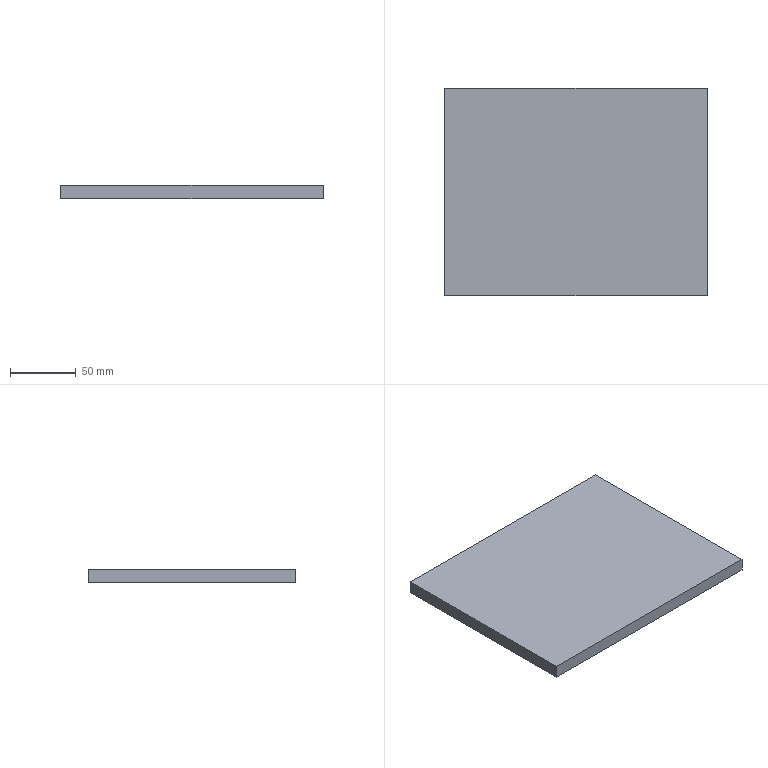Part | NX | features BREP 1 | 1 solid | 6 faces | box 200 x 158 x 10 mm | volume 316000 mm3 | plane 6
STEP:
#1=CARTESIAN_POINT('',(-100.,79.,-5.));
#2=VERTEX_POINT('',#1);
#3=CARTESIAN_POINT('',(-100.,-79.,-5.));
#4=VERTEX_POINT('',#3);
#5=CARTESIAN_POINT('',(-100.,79.,-5.));
#6=DIRECTION('',(0.,-1.,0.));
#7=VECTOR('',#6,1000.);
#8=LINE('',#5,#7);
#9=EDGE_CURVE('',#2,#4,#8,.T.);
#10=ORIENTED_EDGE('',*,*,#9,.T.);
#11=CARTESIAN_POINT('',(-100.,-79.,5.));
#12=VERTEX_POINT('',#11);
#13=CARTESIAN_POINT('',(-100.,-79.,5.));
#14=DIRECTION('',(0.,0.,-1.));
#15=VECTOR('',#14,1000.);
#16=LINE('',#13,#15);
#17=EDGE_CURVE('',#12,#4,#16,.T.);
#18=ORIENTED_EDGE('',*,*,#17,.F.);
#19=CARTESIAN_POINT('',(-100.,79.,5.));
#20=VERTEX_POINT('',#19);
#21=CARTESIAN_POINT('',(-100.,79.,5.));
#22=DIRECTION('',(0.,-1.,0.));
#23=VECTOR('',#22,1000.);
#24=LINE('',#21,#23);
#25=EDGE_CURVE('',#20,#12,#24,.T.);
#26=ORIENTED_EDGE('',*,*,#25,.F.);
#27=CARTESIAN_POINT('',(-100.,79.,5.));
#28=DIRECTION('',(0.,0.,-1.));
#29=VECTOR('',#28,1000.);
#30=LINE('',#27,#29);
#31=EDGE_CURVE('',#20,#2,#30,.T.);
#32=ORIENTED_EDGE('',*,*,#31,.T.);
#33=EDGE_LOOP('',(#10,#18,#26,#32));
#34=FACE_BOUND('',#33,.T.);
#35=CARTESIAN_POINT('',(-100.,79.,5.));
#36=DIRECTION('',(1.,0.,0.));
#37=DIRECTION('',(0.,0.,1.));
#38=AXIS2_PLACEMENT_3D('',#35,#36,#37);
#39=PLANE('',#38);
#40=ADVANCED_FACE('',(#34),#39,.F.);
#41=CARTESIAN_POINT('',(100.,-79.,-5.));
#42=VERTEX_POINT('',#41);
#43=CARTESIAN_POINT('',(-100.,-79.,-5.));
#44=DIRECTION('',(1.,0.,0.));
#45=VECTOR('',#44,1000.);
#46=LINE('',#43,#45);
#47=EDGE_CURVE('',#4,#42,#46,.T.);
#48=ORIENTED_EDGE('',*,*,#47,.T.);
#49=CARTESIAN_POINT('',(100.,-79.,5.));
#50=VERTEX_POINT('',#49);
#51=CARTESIAN_POINT('',(100.,-79.,5.));
#52=DIRECTION('',(0.,0.,-1.));
#53=VECTOR('',#52,1000.);
#54=LINE('',#51,#53);
#55=EDGE_CURVE('',#50,#42,#54,.T.);
#56=ORIENTED_EDGE('',*,*,#55,.F.);
#57=CARTESIAN_POINT('',(-100.,-79.,5.));
#58=DIRECTION('',(1.,0.,0.));
#59=VECTOR('',#58,1000.);
#60=LINE('',#57,#59);
#61=EDGE_CURVE('',#12,#50,#60,.T.);
#62=ORIENTED_EDGE('',*,*,#61,.F.);
#63=ORIENTED_EDGE('',*,*,#17,.T.);
#64=EDGE_LOOP('',(#48,#56,#62,#63));
#65=FACE_BOUND('',#64,.T.);
#66=CARTESIAN_POINT('',(-100.,-79.,5.));
#67=DIRECTION('',(0.,1.,0.));
#68=DIRECTION('',(0.,0.,-1.));
#69=AXIS2_PLACEMENT_3D('',#66,#67,#68);
#70=PLANE('',#69);
#71=ADVANCED_FACE('',(#65),#70,.F.);
#72=CARTESIAN_POINT('',(100.,79.,-5.));
#73=VERTEX_POINT('',#72);
#74=CARTESIAN_POINT('',(100.,79.,-5.));
#75=DIRECTION('',(0.,1.,0.));
#76=VECTOR('',#75,1000.);
#77=LINE('',#74,#76);
#78=EDGE_CURVE('',#42,#73,#77,.T.);
#79=ORIENTED_EDGE('',*,*,#78,.T.);
#80=CARTESIAN_POINT('',(100.,79.,5.));
#81=VERTEX_POINT('',#80);
#82=CARTESIAN_POINT('',(100.,79.,5.));
#83=DIRECTION('',(0.,0.,-1.));
#84=VECTOR('',#83,1000.);
#85=LINE('',#82,#84);
#86=EDGE_CURVE('',#81,#73,#85,.T.);
#87=ORIENTED_EDGE('',*,*,#86,.F.);
#88=CARTESIAN_POINT('',(100.,79.,5.));
#89=DIRECTION('',(0.,1.,0.));
#90=VECTOR('',#89,1000.);
#91=LINE('',#88,#90);
#92=EDGE_CURVE('',#50,#81,#91,.T.);
#93=ORIENTED_EDGE('',*,*,#92,.F.);
#94=ORIENTED_EDGE('',*,*,#55,.T.);
#95=EDGE_LOOP('',(#79,#87,#93,#94));
#96=FACE_BOUND('',#95,.T.);
#97=CARTESIAN_POINT('',(100.,79.,5.));
#98=DIRECTION('',(-1.,0.,0.));
#99=DIRECTION('',(0.,0.,-1.));
#100=AXIS2_PLACEMENT_3D('',#97,#98,#99);
#101=PLANE('',#100);
#102=ADVANCED_FACE('',(#96),#101,.F.);
#103=CARTESIAN_POINT('',(-100.,79.,-5.));
#104=DIRECTION('',(-1.,0.,0.));
#105=VECTOR('',#104,1000.);
#106=LINE('',#103,#105);
#107=EDGE_CURVE('',#73,#2,#106,.T.);
#108=ORIENTED_EDGE('',*,*,#107,.T.);
#109=ORIENTED_EDGE('',*,*,#31,.F.);
#110=CARTESIAN_POINT('',(-100.,79.,5.));
#111=DIRECTION('',(-1.,0.,0.));
#112=VECTOR('',#111,1000.);
#113=LINE('',#110,#112);
#114=EDGE_CURVE('',#81,#20,#113,.T.);
#115=ORIENTED_EDGE('',*,*,#114,.F.);
#116=ORIENTED_EDGE('',*,*,#86,.T.);
#117=EDGE_LOOP('',(#108,#109,#115,#116));
#118=FACE_BOUND('',#117,.T.);
#119=CARTESIAN_POINT('',(-100.,79.,5.));
#120=DIRECTION('',(0.,-1.,0.));
#121=DIRECTION('',(0.,0.,1.));
#122=AXIS2_PLACEMENT_3D('',#119,#120,#121);
#123=PLANE('',#122);
#124=ADVANCED_FACE('',(#118),#123,.F.);
#125=ORIENTED_EDGE('',*,*,#25,.T.);
#126=ORIENTED_EDGE('',*,*,#61,.T.);
#127=ORIENTED_EDGE('',*,*,#92,.T.);
#128=ORIENTED_EDGE('',*,*,#114,.T.);
#129=EDGE_LOOP('',(#125,#126,#127,#128));
#130=FACE_BOUND('',#129,.T.);
#131=CARTESIAN_POINT('',(-100.,-79.,5.));
#132=DIRECTION('',(0.,0.,1.));
#133=DIRECTION('',(-1.,0.,0.));
#134=AXIS2_PLACEMENT_3D('',#131,#132,#133);
#135=PLANE('',#134);
#136=ADVANCED_FACE('',(#130),#135,.T.);
#137=ORIENTED_EDGE('',*,*,#9,.F.);
#138=ORIENTED_EDGE('',*,*,#107,.F.);
#139=ORIENTED_EDGE('',*,*,#78,.F.);
#140=ORIENTED_EDGE('',*,*,#47,.F.);
#141=EDGE_LOOP('',(#137,#138,#139,#140));
#142=FACE_BOUND('',#141,.T.);
#143=CARTESIAN_POINT('',(-100.,-79.,-5.));
#144=DIRECTION('',(0.,0.,1.));
#145=DIRECTION('',(-1.,0.,0.));
#146=AXIS2_PLACEMENT_3D('',#143,#144,#145);
#147=PLANE('',#146);
#148=ADVANCED_FACE('',(#142),#147,.F.);
#149=CLOSED_SHELL('',(#40,#71,#102,#124,#136,#148));
#150=MANIFOLD_SOLID_BREP('',#149);
#151=(LENGTH_UNIT()NAMED_UNIT(*)SI_UNIT(.MILLI.,.METRE.));
#152=UNCERTAINTY_MEASURE_WITH_UNIT(LENGTH_MEASURE(0.00001),#151,'','');
#153=(NAMED_UNIT(*)PLANE_ANGLE_UNIT()SI_UNIT($,.RADIAN.));
#154=(NAMED_UNIT(*)SI_UNIT($,.STERADIAN.)SOLID_ANGLE_UNIT());
#155=(GEOMETRIC_REPRESENTATION_CONTEXT(3)GLOBAL_UNCERTAINTY_ASSIGNED_CONTEXT((#152))GLOBAL_UNIT_ASSIGNED_CONTEXT((#151,#153,#154))REPRESENTATION_CONTEXT('',''));
#156=ADVANCED_BREP_SHAPE_REPRESENTATION('',(#150),#155);